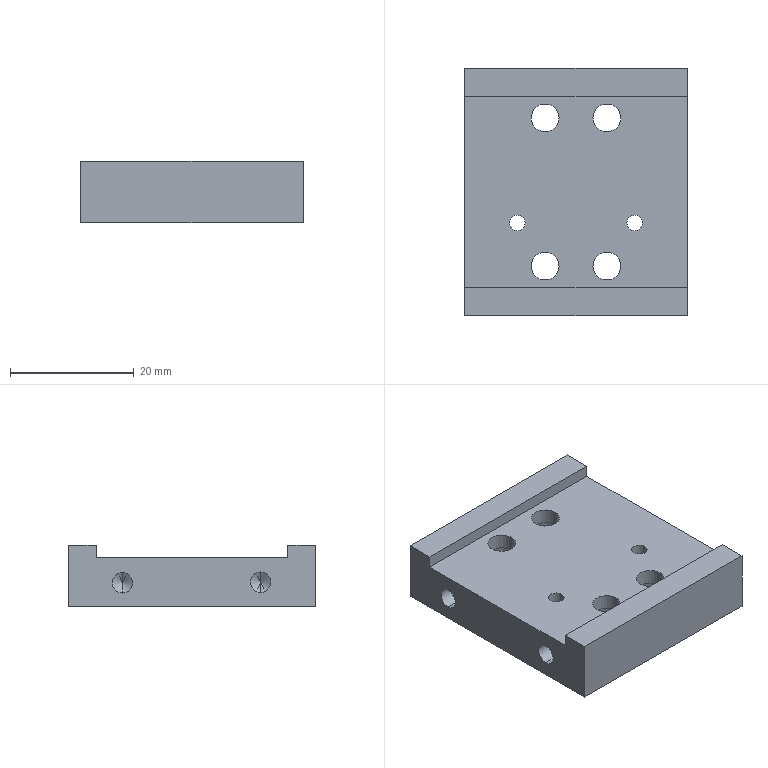Part | STEP file | Slide cylinder mount | 1 solid | 42 faces | box 36 x 40 x 10 mm | volume 10816 mm3 | cylinder 24 | plane 14 | cone 4 | commonest cylinder face diameters 4.5 x8 7.5 x8 2.5 x4 3.3 x4